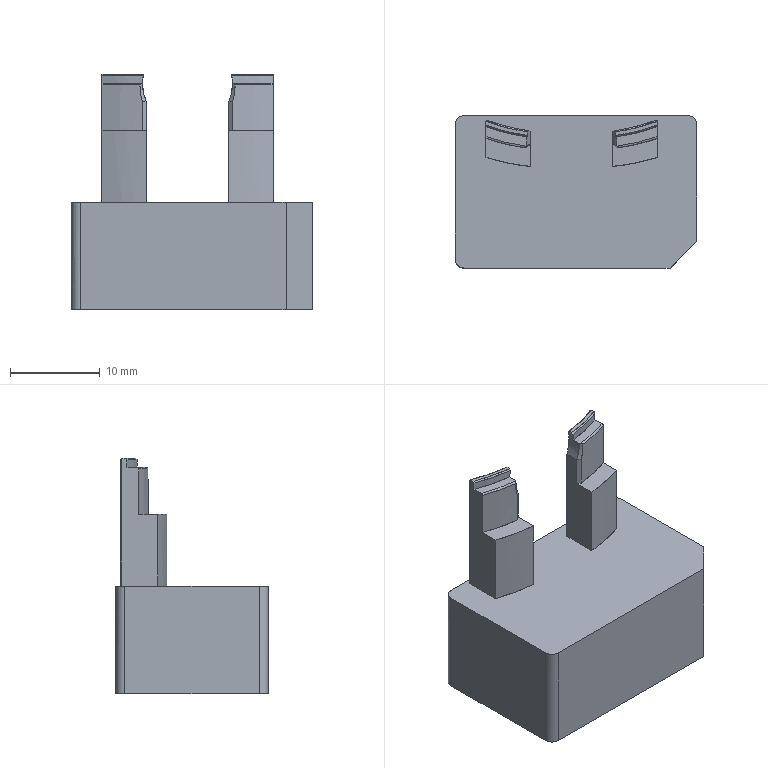CAM job | PowerMill | 3-axis milling, other | part box 27 x 17 x 26.255 mm
Tools:
number,name,type,diameter,tip_radius,length,cutting_length,overhang,flutes,holder,toolpaths_using
1,D10C,end_mill,10.0,0.0,60.0,,30.0,1,D42L35,1
1,D10C_1_1_1,end_mill,10.0,0.0,60.0,,26.72,1,D42L35,3
15,D3C_1_1,end_mill,3.0,0.0,30.0,,14.44,1,D42L35,1
3,D10_1_1_1,end_mill,10.0,0.0,60.0,,26.4,1,D42L35,3
10,D3_1_1,end_mill,3.0,0.0,30.0,,14.4,1,D42L35,2
13,Text_D4_1_1,taper_spherical,4.0,0.3,60.0,,14.52,1,D42L35,1
Operations:
program,toolpath,strategy,tool,tool_number,tool_diameter,tip_radius,flutes,spindle_rpm,feed_cut,surface_speed_m_min_computed,feed_per_tooth_computed,tolerance,thickness,stepover,stepdown,cut_length,cut_time_min,total_time_min,workplane
006-0610-4-F,精公开粗01-扫面平行-D10C,raster_area_clear,D10C_1_1_1,1,10.0,0.0,1.0,8000.0,10000.0,251.33,1.25,0.03,0.28,6.0,1.0,185.36,0.018,0.0241,
006-0610-4-F,精公开粗01-外形偏置-D10C,offset_area_clear,D10C_1_1_1,1,10.0,0.0,1.0,8000.0,10000.0,251.33,1.25,0.03,0.28,6.0,1.0,9095.174,0.909,1.002,
006-0610-4-F,精公开粗01-基准台等高-D10C,constantz,D10C_1_1_1,1,10.0,0.0,1.0,8000.0,10000.0,251.33,1.25,0.03,0.07,5.0,0.4,3736.815,0.374,0.3843,
006-0610-4-F,精公再粗02-外形偏置-D3C,offset_area_clear,D3C_1_1,15,3.0,0.0,1.0,18000.0,5000.0,169.65,0.2778,0.03,0.0,2.0,1.0,5820.606,1.164,1.639,
006-0610-4-F,精公基准台01-平坦面平行-D10,raster_area_clear,D10_1_1_1,3,10.0,0.0,1.0,8500.0,600.0,267.04,0.0706,0.005,0.38,5.0,1.0,206.922,0.345,0.4335,
006-0610-4-F,精公基准台01-基准面偏置-D10,offset_area_clear,D10_1_1_1,3,10.0,0.0,1.0,8500.0,600.0,267.04,0.0706,0.005,0.38,5.0,1.0,153.723,0.256,0.2752,
006-0610-4-F,精公基准台01-基准台侧光-D10,profile_area_clear,D10_1_1_1,3,10.0,0.0,1.0,8500.0,600.0,267.04,0.0706,0.005,0.0,0.08,1.0,233.233,0.389,0.454,
006-0610-4-F,精公精光01-等高-D3,constantz,D3_1_1,10,3.0,0.0,1.0,18000.0,2000.0,169.65,0.1111,0.005,-0.075,5.0,0.02,16619.462,8.31,9.164,
006-0610-4-F,精公精光01-平坦面平行-D3,raster_area_clear,D3_1_1,10,3.0,0.0,1.0,18000.0,600.0,169.65,0.0333,0.005,0.375,1.5,1.0,164.775,0.275,0.3591,
006-0610-4-F,精公刻字01-刻字-Text_D4,pattern,Text_D4_1_1,13,4.0,0.3,1.0,15000.0,1000.0,188.5,0.0667,0.005,0.0,5.0,1.0,48.804,0.049,0.0686,
,精公开粗01-外形偏置-D10C_Reference,offset_area_clear,D10C,1,10.0,0.0,1.0,8000.0,10000.0,251.33,1.25,0.03,0.28,6.0,1.0,23257.746,2.326,2.559,